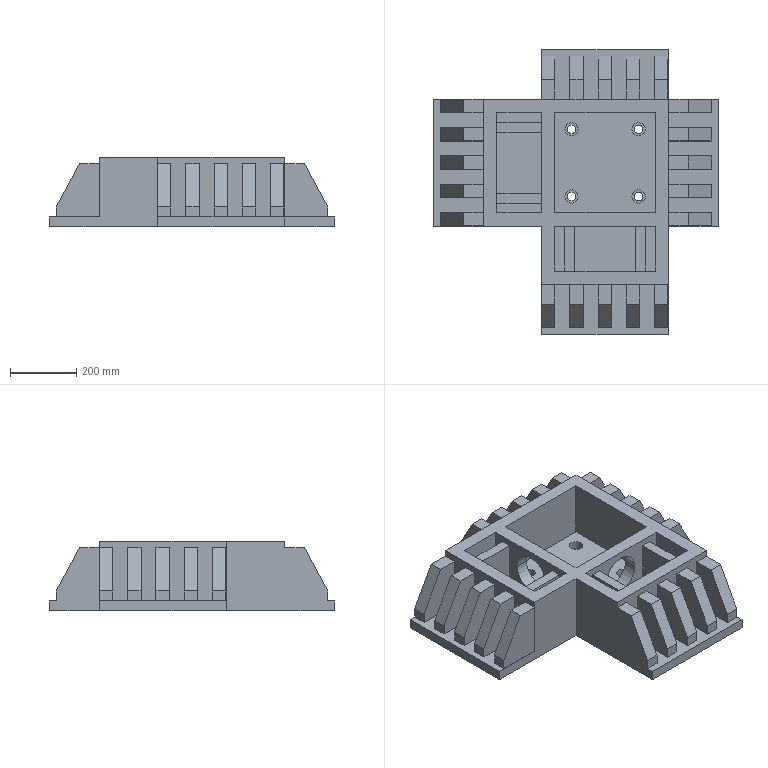Part | SolidWorks | features ICE 11, Extrusion 1 | 1 solid | 170 faces | box 857 x 857 x 210 mm | volume 50598262 mm3 | plane 150 | cylinder 20 | commonest cylinder face diameters 26 x8 40 x8 120 x4